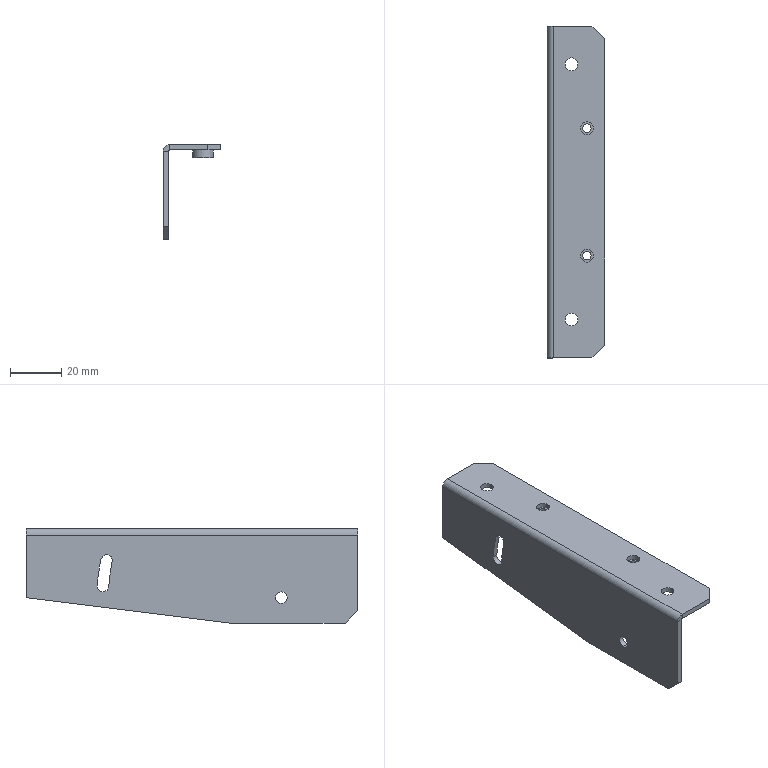Part | SolidWorks | features ICE 3, Chamfer 2, Cut 2, FlatPattern 1, HoleWzd 1, SMBaseFlange 1, SheetMetal 1 | 1 solid | 45 faces | box 22.5 x 130 x 37 mm | volume 13846 mm3 | cylinder 25 | plane 20 | commonest cylinder face diameters 5 x9 4.5 x5 3.3 x4 8 x4 1 x1 135.5 x1
STEP:
#1=CARTESIAN_POINT('',(15.15,40.,-3.));
#2=VERTEX_POINT('',#1);
#3=CARTESIAN_POINT('',(11.85,40.,-3.));
#4=VERTEX_POINT('',#3);
#5=CARTESIAN_POINT('',(13.5,40.,-3.));
#6=DIRECTION('',(0.,0.,-1.));
#7=DIRECTION('',(-1.,0.,0.));
#8=AXIS2_PLACEMENT_3D('',#5,#6,#7);
#9=CIRCLE('',#8,1.65);
#10=EDGE_CURVE('',#2,#4,#9,.T.);
#11=ORIENTED_EDGE('',*,*,#10,.T.);
#12=CARTESIAN_POINT('',(11.85,40.,0.));
#13=VERTEX_POINT('',#12);
#14=CARTESIAN_POINT('',(11.85,40.,0.));
#15=DIRECTION('',(0.,0.,1.));
#16=VECTOR('',#15,1000.);
#17=LINE('',#14,#16);
#18=EDGE_CURVE('',#4,#13,#17,.T.);
#19=ORIENTED_EDGE('',*,*,#18,.T.);
#20=CARTESIAN_POINT('',(15.15,40.,0.));
#21=VERTEX_POINT('',#20);
#22=CARTESIAN_POINT('',(13.5,40.,0.));
#23=DIRECTION('',(0.,0.,1.));
#24=DIRECTION('',(1.,0.,0.));
#25=AXIS2_PLACEMENT_3D('',#22,#23,#24);
#26=CIRCLE('',#25,1.65);
#27=EDGE_CURVE('',#13,#21,#26,.T.);
#28=ORIENTED_EDGE('',*,*,#27,.T.);
#29=CARTESIAN_POINT('',(15.15,40.,0.));
#30=DIRECTION('',(0.,0.,1.));
#31=VECTOR('',#30,1000.);
#32=LINE('',#29,#31);
#33=EDGE_CURVE('',#2,#21,#32,.T.);
#34=ORIENTED_EDGE('',*,*,#33,.F.);
#35=EDGE_LOOP('',(#11,#19,#28,#34));
#36=FACE_OUTER_BOUND('',#35,.T.);
#37=CARTESIAN_POINT('',(13.5,40.,0.));
#38=DIRECTION('',(0.,0.,1.));
#39=DIRECTION('',(1.,0.,0.));
#40=AXIS2_PLACEMENT_3D('',#37,#38,#39);
#41=CYLINDRICAL_SURFACE('',#40,1.65);
#42=ADVANCED_FACE('',(#36),#41,.F.);
#43=CARTESIAN_POINT('',(15.15,90.,-3.));
#44=VERTEX_POINT('',#43);
#45=CARTESIAN_POINT('',(11.85,90.,-3.));
#46=VERTEX_POINT('',#45);
#47=CARTESIAN_POINT('',(13.5,90.,-3.));
#48=DIRECTION('',(0.,0.,-1.));
#49=DIRECTION('',(-1.,0.,0.));
#50=AXIS2_PLACEMENT_3D('',#47,#48,#49);
#51=CIRCLE('',#50,1.65);
#52=EDGE_CURVE('',#44,#46,#51,.T.);
#53=ORIENTED_EDGE('',*,*,#52,.T.);
#54=CARTESIAN_POINT('',(11.85,90.,0.));
#55=VERTEX_POINT('',#54);
#56=CARTESIAN_POINT('',(11.85,90.,0.));
#57=DIRECTION('',(0.,0.,1.));
#58=VECTOR('',#57,1000.);
#59=LINE('',#56,#58);
#60=EDGE_CURVE('',#46,#55,#59,.T.);
#61=ORIENTED_EDGE('',*,*,#60,.T.);
#62=CARTESIAN_POINT('',(15.15,90.,0.));
#63=VERTEX_POINT('',#62);
#64=CARTESIAN_POINT('',(13.5,90.,0.));
#65=DIRECTION('',(0.,0.,1.));
#66=DIRECTION('',(1.,0.,0.));
#67=AXIS2_PLACEMENT_3D('',#64,#65,#66);
#68=CIRCLE('',#67,1.65);
#69=EDGE_CURVE('',#55,#63,#68,.T.);
#70=ORIENTED_EDGE('',*,*,#69,.T.);
#71=CARTESIAN_POINT('',(15.15,90.,0.));
#72=DIRECTION('',(0.,0.,1.));
#73=VECTOR('',#72,1000.);
#74=LINE('',#71,#73);
#75=EDGE_CURVE('',#44,#63,#74,.T.);
#76=ORIENTED_EDGE('',*,*,#75,.F.);
#77=EDGE_LOOP('',(#53,#61,#70,#76));
#78=FACE_OUTER_BOUND('',#77,.T.);
#79=CARTESIAN_POINT('',(13.5,90.,0.));
#80=DIRECTION('',(0.,0.,1.));
#81=DIRECTION('',(1.,0.,0.));
#82=AXIS2_PLACEMENT_3D('',#79,#80,#81);
#83=CYLINDRICAL_SURFACE('',#82,1.65);
#84=ADVANCED_FACE('',(#78),#83,.F.);
#85=CARTESIAN_POINT('',(9.5,90.,-3.));
#86=VERTEX_POINT('',#85);
#87=CARTESIAN_POINT('',(17.5,90.,-3.));
#88=VERTEX_POINT('',#87);
#89=CARTESIAN_POINT('',(13.5,90.,-3.));
#90=DIRECTION('',(0.,0.,-1.));
#91=DIRECTION('',(-1.,0.,0.));
#92=AXIS2_PLACEMENT_3D('',#89,#90,#91);
#93=CIRCLE('',#92,4.);
#94=EDGE_CURVE('',#86,#88,#93,.T.);
#95=ORIENTED_EDGE('',*,*,#94,.F.);
#96=CARTESIAN_POINT('',(9.5,90.,0.));
#97=VERTEX_POINT('',#96);
#98=CARTESIAN_POINT('',(9.5,90.,-3.));
#99=DIRECTION('',(0.,0.,1.));
#100=VECTOR('',#99,1000.);
#101=LINE('',#98,#100);
#102=EDGE_CURVE('',#86,#97,#101,.T.);
#103=ORIENTED_EDGE('',*,*,#102,.T.);
#104=CARTESIAN_POINT('',(17.5,90.,0.));
#105=VERTEX_POINT('',#104);
#106=CARTESIAN_POINT('',(13.5,90.,0.));
#107=DIRECTION('',(0.,0.,-1.));
#108=DIRECTION('',(-1.,0.,0.));
#109=AXIS2_PLACEMENT_3D('',#106,#107,#108);
#110=CIRCLE('',#109,4.);
#111=EDGE_CURVE('',#97,#105,#110,.T.);
#112=ORIENTED_EDGE('',*,*,#111,.T.);
#113=CARTESIAN_POINT('',(17.5,90.,-3.));
#114=DIRECTION('',(0.,0.,1.));
#115=VECTOR('',#114,1000.);
#116=LINE('',#113,#115);
#117=EDGE_CURVE('',#88,#105,#116,.T.);
#118=ORIENTED_EDGE('',*,*,#117,.F.);
#119=EDGE_LOOP('',(#95,#103,#112,#118));
#120=FACE_OUTER_BOUND('',#119,.T.);
#121=CARTESIAN_POINT('',(13.5,90.,-3.));
#122=DIRECTION('',(0.,0.,1.));
#123=DIRECTION('',(1.,0.,0.));
#124=AXIS2_PLACEMENT_3D('',#121,#122,#123);
#125=CYLINDRICAL_SURFACE('',#124,4.);
#126=ADVANCED_FACE('',(#120),#125,.T.);
#127=CARTESIAN_POINT('',(9.5,40.,-3.));
#128=VERTEX_POINT('',#127);
#129=CARTESIAN_POINT('',(17.5,40.,-3.));
#130=VERTEX_POINT('',#129);
#131=CARTESIAN_POINT('',(13.5,40.,-3.));
#132=DIRECTION('',(0.,0.,-1.));
#133=DIRECTION('',(-1.,0.,0.));
#134=AXIS2_PLACEMENT_3D('',#131,#132,#133);
#135=CIRCLE('',#134,4.);
#136=EDGE_CURVE('',#128,#130,#135,.T.);
#137=ORIENTED_EDGE('',*,*,#136,.F.);
#138=CARTESIAN_POINT('',(9.5,40.,0.));
#139=VERTEX_POINT('',#138);
#140=CARTESIAN_POINT('',(9.5,40.,-3.));
#141=DIRECTION('',(0.,0.,1.));
#142=VECTOR('',#141,1000.);
#143=LINE('',#140,#142);
#144=EDGE_CURVE('',#128,#139,#143,.T.);
#145=ORIENTED_EDGE('',*,*,#144,.T.);
#146=CARTESIAN_POINT('',(17.5,40.,0.));
#147=VERTEX_POINT('',#146);
#148=CARTESIAN_POINT('',(13.5,40.,0.));
#149=DIRECTION('',(0.,0.,-1.));
#150=DIRECTION('',(-1.,0.,0.));
#151=AXIS2_PLACEMENT_3D('',#148,#149,#150);
#152=CIRCLE('',#151,4.);
#153=EDGE_CURVE('',#139,#147,#152,.T.);
#154=ORIENTED_EDGE('',*,*,#153,.T.);
#155=CARTESIAN_POINT('',(17.5,40.,-3.));
#156=DIRECTION('',(0.,0.,1.));
#157=VECTOR('',#156,1000.);
#158=LINE('',#155,#157);
#159=EDGE_CURVE('',#130,#147,#158,.T.);
#160=ORIENTED_EDGE('',*,*,#159,.F.);
#161=EDGE_LOOP('',(#137,#145,#154,#160));
#162=FACE_OUTER_BOUND('',#161,.T.);
#163=CARTESIAN_POINT('',(13.5,40.,-3.));
#164=DIRECTION('',(0.,0.,1.));
#165=DIRECTION('',(1.,0.,0.));
#166=AXIS2_PLACEMENT_3D('',#163,#164,#165);
#167=CYLINDRICAL_SURFACE('',#166,4.);
#168=ADVANCED_FACE('',(#162),#167,.T.);
#169=CARTESIAN_POINT('',(16.,40.,2.));
#170=VERTEX_POINT('',#169);
#171=CARTESIAN_POINT('',(11.,40.,2.));
#172=VERTEX_POINT('',#171);
#173=CARTESIAN_POINT('',(13.5,40.,2.));
#174=DIRECTION('',(0.,0.,-1.));
#175=DIRECTION('',(-1.,0.,0.));
#176=AXIS2_PLACEMENT_3D('',#173,#174,#175);
#177=CIRCLE('',#176,2.5);
#178=EDGE_CURVE('',#170,#172,#177,.T.);
#179=ORIENTED_EDGE('',*,*,#178,.F.);
#180=CARTESIAN_POINT('',(16.,40.,0.));
#181=VERTEX_POINT('',#180);
#182=CARTESIAN_POINT('',(16.,40.,5.));
#183=DIRECTION('',(0.,0.,-1.));
#184=VECTOR('',#183,1000.);
#185=LINE('',#182,#184);
#186=EDGE_CURVE('',#170,#181,#185,.T.);
#187=ORIENTED_EDGE('',*,*,#186,.T.);
#188=CARTESIAN_POINT('',(11.,40.,0.));
#189=VERTEX_POINT('',#188);
#190=CARTESIAN_POINT('',(13.5,40.,0.));
#191=DIRECTION('',(0.,0.,1.));
#192=DIRECTION('',(-1.,0.,0.));
#193=AXIS2_PLACEMENT_3D('',#190,#191,#192);
#194=CIRCLE('',#193,2.5);
#195=EDGE_CURVE('',#189,#181,#194,.T.);
#196=ORIENTED_EDGE('',*,*,#195,.F.);
#197=CARTESIAN_POINT('',(11.,40.,5.));
#198=DIRECTION('',(0.,0.,-1.));
#199=VECTOR('',#198,1000.);
#200=LINE('',#197,#199);
#201=EDGE_CURVE('',#172,#189,#200,.T.);
#202=ORIENTED_EDGE('',*,*,#201,.F.);
#203=EDGE_LOOP('',(#179,#187,#196,#202));
#204=FACE_OUTER_BOUND('',#203,.T.);
#205=CARTESIAN_POINT('',(13.5,40.,5.));
#206=DIRECTION('',(0.,0.,-1.));
#207=DIRECTION('',(-1.,0.,0.));
#208=AXIS2_PLACEMENT_3D('',#205,#206,#207);
#209=CYLINDRICAL_SURFACE('',#208,2.5);
#210=ADVANCED_FACE('',(#204),#209,.F.);
#211=CARTESIAN_POINT('',(16.,90.,2.));
#212=VERTEX_POINT('',#211);
#213=CARTESIAN_POINT('',(11.,90.,2.));
#214=VERTEX_POINT('',#213);
#215=CARTESIAN_POINT('',(13.5,90.,2.));
#216=DIRECTION('',(0.,0.,-1.));
#217=DIRECTION('',(-1.,0.,0.));
#218=AXIS2_PLACEMENT_3D('',#215,#216,#217);
#219=CIRCLE('',#218,2.5);
#220=EDGE_CURVE('',#212,#214,#219,.T.);
#221=ORIENTED_EDGE('',*,*,#220,.F.);
#222=CARTESIAN_POINT('',(16.,90.,0.));
#223=VERTEX_POINT('',#222);
#224=CARTESIAN_POINT('',(16.,90.,5.));
#225=DIRECTION('',(0.,0.,-1.));
#226=VECTOR('',#225,1000.);
#227=LINE('',#224,#226);
#228=EDGE_CURVE('',#212,#223,#227,.T.);
#229=ORIENTED_EDGE('',*,*,#228,.T.);
#230=CARTESIAN_POINT('',(11.,90.,0.));
#231=VERTEX_POINT('',#230);
#232=CARTESIAN_POINT('',(13.5,90.,0.));
#233=DIRECTION('',(0.,0.,1.));
#234=DIRECTION('',(-1.,0.,0.));
#235=AXIS2_PLACEMENT_3D('',#232,#233,#234);
#236=CIRCLE('',#235,2.5);
#237=EDGE_CURVE('',#231,#223,#236,.T.);
#238=ORIENTED_EDGE('',*,*,#237,.F.);
#239=CARTESIAN_POINT('',(11.,90.,5.));
#240=DIRECTION('',(0.,0.,-1.));
#241=VECTOR('',#240,1000.);
#242=LINE('',#239,#241);
#243=EDGE_CURVE('',#214,#231,#242,.T.);
#244=ORIENTED_EDGE('',*,*,#243,.F.);
#245=EDGE_LOOP('',(#221,#229,#238,#244));
#246=FACE_OUTER_BOUND('',#245,.T.);
#247=CARTESIAN_POINT('',(13.5,90.,5.));
#248=DIRECTION('',(0.,0.,-1.));
#249=DIRECTION('',(-1.,0.,0.));
#250=AXIS2_PLACEMENT_3D('',#247,#248,#249);
#251=CYLINDRICAL_SURFACE('',#250,2.5);
#252=ADVANCED_FACE('',(#246),#251,.F.);
#253=CARTESIAN_POINT('',(0.,100.671,-9.978));
#254=VERTEX_POINT('',#253);
#255=CARTESIAN_POINT('',(0.,98.47,-8.196));
#256=VERTEX_POINT('',#255);
#257=CARTESIAN_POINT('',(0.,98.47,-10.446));
#258=DIRECTION('',(1.,0.,0.));
#259=DIRECTION('',(0.,0.,-1.));
#260=AXIS2_PLACEMENT_3D('',#257,#258,#259);
#261=CIRCLE('',#260,2.25);
#262=EDGE_CURVE('',#254,#256,#261,.T.);
#263=ORIENTED_EDGE('',*,*,#262,.T.);
#264=CARTESIAN_POINT('',(-2.,98.47,-8.196));
#265=VERTEX_POINT('',#264);
#266=CARTESIAN_POINT('',(8.,98.47,-8.196));
#267=DIRECTION('',(-1.,0.,0.));
#268=VECTOR('',#267,1000.);
#269=LINE('',#266,#268);
#270=EDGE_CURVE('',#256,#265,#269,.T.);
#271=ORIENTED_EDGE('',*,*,#270,.T.);
#272=CARTESIAN_POINT('',(-2.,100.671,-9.978));
#273=VERTEX_POINT('',#272);
#274=CARTESIAN_POINT('',(-2.,98.47,-10.446));
#275=DIRECTION('',(-1.,0.,0.));
#276=DIRECTION('',(0.,0.,1.));
#277=AXIS2_PLACEMENT_3D('',#274,#275,#276);
#278=CIRCLE('',#277,2.25);
#279=EDGE_CURVE('',#265,#273,#278,.T.);
#280=ORIENTED_EDGE('',*,*,#279,.T.);
#281=CARTESIAN_POINT('',(8.,100.671,-9.978));
#282=DIRECTION('',(-1.,0.,0.));
#283=VECTOR('',#282,1000.);
#284=LINE('',#281,#283);
#285=EDGE_CURVE('',#254,#273,#284,.T.);
#286=ORIENTED_EDGE('',*,*,#285,.F.);
#287=EDGE_LOOP('',(#263,#271,#280,#286));
#288=FACE_OUTER_BOUND('',#287,.T.);
#289=CARTESIAN_POINT('',(8.,98.47,-10.446));
#290=DIRECTION('',(-1.,0.,0.));
#291=DIRECTION('',(0.,0.,1.));
#292=AXIS2_PLACEMENT_3D('',#289,#290,#291);
#293=CYLINDRICAL_SURFACE('',#292,2.25);
#294=ADVANCED_FACE('',(#288),#293,.F.);
#295=CARTESIAN_POINT('',(-2.,30.,-22.75));
#296=VERTEX_POINT('',#295);
#297=CARTESIAN_POINT('',(-2.,30.,-27.25));
#298=VERTEX_POINT('',#297);
#299=CARTESIAN_POINT('',(-2.,30.,-25.));
#300=DIRECTION('',(1.,0.,0.));
#301=DIRECTION('',(0.,0.,-1.));
#302=AXIS2_PLACEMENT_3D('',#299,#300,#301);
#303=CIRCLE('',#302,2.25);
#304=EDGE_CURVE('',#296,#298,#303,.T.);
#305=ORIENTED_EDGE('',*,*,#304,.F.);
#306=CARTESIAN_POINT('',(0.,30.,-22.75));
#307=VERTEX_POINT('',#306);
#308=CARTESIAN_POINT('',(-10.,30.,-22.75));
#309=DIRECTION('',(1.,0.,0.));
#310=VECTOR('',#309,1000.);
#311=LINE('',#308,#310);
#312=EDGE_CURVE('',#296,#307,#311,.T.);
#313=ORIENTED_EDGE('',*,*,#312,.T.);
#314=CARTESIAN_POINT('',(0.,30.,-27.25));
#315=VERTEX_POINT('',#314);
#316=CARTESIAN_POINT('',(0.,30.,-25.));
#317=DIRECTION('',(1.,0.,0.));
#318=DIRECTION('',(0.,0.,-1.));
#319=AXIS2_PLACEMENT_3D('',#316,#317,#318);
#320=CIRCLE('',#319,2.25);
#321=EDGE_CURVE('',#307,#315,#320,.T.);
#322=ORIENTED_EDGE('',*,*,#321,.T.);
#323=CARTESIAN_POINT('',(-10.,30.,-27.25));
#324=DIRECTION('',(1.,0.,0.));
#325=VECTOR('',#324,1000.);
#326=LINE('',#323,#325);
#327=EDGE_CURVE('',#298,#315,#326,.T.);
#328=ORIENTED_EDGE('',*,*,#327,.F.);
#329=EDGE_LOOP('',(#305,#313,#322,#328));
#330=FACE_OUTER_BOUND('',#329,.T.);
#331=CARTESIAN_POINT('',(-10.,30.,-25.));
#332=DIRECTION('',(1.,0.,0.));
#333=DIRECTION('',(0.,0.,-1.));
#334=AXIS2_PLACEMENT_3D('',#331,#332,#333);
#335=CYLINDRICAL_SURFACE('',#334,2.25);
#336=ADVANCED_FACE('',(#330),#335,.F.);
#337=CARTESIAN_POINT('',(10.,15.,0.));
#338=VERTEX_POINT('',#337);
#339=CARTESIAN_POINT('',(5.,15.,0.));
#340=VERTEX_POINT('',#339);
#341=CARTESIAN_POINT('',(7.5,15.,0.));
#342=DIRECTION('',(0.,0.,-1.));
#343=DIRECTION('',(-1.,0.,0.));
#344=AXIS2_PLACEMENT_3D('',#341,#342,#343);
#345=CIRCLE('',#344,2.5);
#346=EDGE_CURVE('',#338,#340,#345,.T.);
#347=ORIENTED_EDGE('',*,*,#346,.T.);
#348=CARTESIAN_POINT('',(5.,15.,2.));
#349=VERTEX_POINT('',#348);
#350=CARTESIAN_POINT('',(5.,15.,-8.));
#351=DIRECTION('',(0.,0.,1.));
#352=VECTOR('',#351,1000.);
#353=LINE('',#350,#352);
#354=EDGE_CURVE('',#340,#349,#353,.T.);
#355=ORIENTED_EDGE('',*,*,#354,.T.);
#356=CARTESIAN_POINT('',(10.,15.,2.));
#357=VERTEX_POINT('',#356);
#358=CARTESIAN_POINT('',(7.5,15.,2.));
#359=DIRECTION('',(0.,0.,1.));
#360=DIRECTION('',(1.,0.,0.));
#361=AXIS2_PLACEMENT_3D('',#358,#359,#360);
#362=CIRCLE('',#361,2.5);
#363=EDGE_CURVE('',#349,#357,#362,.T.);
#364=ORIENTED_EDGE('',*,*,#363,.T.);
#365=CARTESIAN_POINT('',(10.,15.,-8.));
#366=DIRECTION('',(0.,0.,1.));
#367=VECTOR('',#366,1000.);
#368=LINE('',#365,#367);
#369=EDGE_CURVE('',#338,#357,#368,.T.);
#370=ORIENTED_EDGE('',*,*,#369,.F.);
#371=EDGE_LOOP('',(#347,#355,#364,#370));
#372=FACE_OUTER_BOUND('',#371,.T.);
#373=CARTESIAN_POINT('',(7.5,15.,-8.));
#374=DIRECTION('',(0.,0.,1.));
#375=DIRECTION('',(1.,0.,0.));
#376=AXIS2_PLACEMENT_3D('',#373,#374,#375);
#377=CYLINDRICAL_SURFACE('',#376,2.5);
#378=ADVANCED_FACE('',(#372),#377,.F.);
#379=CARTESIAN_POINT('',(10.,115.,0.));
#380=VERTEX_POINT('',#379);
#381=CARTESIAN_POINT('',(5.,115.,0.));
#382=VERTEX_POINT('',#381);
#383=CARTESIAN_POINT('',(7.5,115.,0.));
#384=DIRECTION('',(0.,0.,-1.));
#385=DIRECTION('',(-1.,0.,0.));
#386=AXIS2_PLACEMENT_3D('',#383,#384,#385);
#387=CIRCLE('',#386,2.5);
#388=EDGE_CURVE('',#380,#382,#387,.T.);
#389=ORIENTED_EDGE('',*,*,#388,.T.);
#390=CARTESIAN_POINT('',(5.,115.,2.));
#391=VERTEX_POINT('',#390);
#392=CARTESIAN_POINT('',(5.,115.,-8.));
#393=DIRECTION('',(0.,0.,1.));
#394=VECTOR('',#393,1000.);
#395=LINE('',#392,#394);
#396=EDGE_CURVE('',#382,#391,#395,.T.);
#397=ORIENTED_EDGE('',*,*,#396,.T.);
#398=CARTESIAN_POINT('',(10.,115.,2.));
#399=VERTEX_POINT('',#398);
#400=CARTESIAN_POINT('',(7.5,115.,2.));
#401=DIRECTION('',(0.,0.,1.));
#402=DIRECTION('',(1.,0.,0.));
#403=AXIS2_PLACEMENT_3D('',#400,#401,#402);
#404=CIRCLE('',#403,2.5);
#405=EDGE_CURVE('',#391,#399,#404,.T.);
#406=ORIENTED_EDGE('',*,*,#405,.T.);
#407=CARTESIAN_POINT('',(10.,115.,-8.));
#408=DIRECTION('',(0.,0.,1.));
#409=VECTOR('',#408,1000.);
#410=LINE('',#407,#409);
#411=EDGE_CURVE('',#380,#399,#410,.T.);
#412=ORIENTED_EDGE('',*,*,#411,.F.);
#413=EDGE_LOOP('',(#389,#397,#406,#412));
#414=FACE_OUTER_BOUND('',#413,.T.);
#415=CARTESIAN_POINT('',(7.5,115.,-8.));
#416=DIRECTION('',(0.,0.,1.));
#417=DIRECTION('',(1.,0.,0.));
#418=AXIS2_PLACEMENT_3D('',#415,#416,#417);
#419=CYLINDRICAL_SURFACE('',#418,2.5);
#420=ADVANCED_FACE('',(#414),#419,.F.);
#421=CARTESIAN_POINT('',(13.5,40.,0.));
#422=DIRECTION('',(0.,0.,-1.));
#423=DIRECTION('',(-1.,0.,0.));
#424=AXIS2_PLACEMENT_3D('',#421,#422,#423);
#425=CIRCLE('',#424,4.);
#426=EDGE_CURVE('',#147,#139,#425,.T.);
#427=ORIENTED_EDGE('',*,*,#426,.F.);
#428=ORIENTED_EDGE('',*,*,#153,.F.);
#429=EDGE_LOOP('',(#427,#428));
#430=FACE_BOUND('',#429,.T.);
#431=ORIENTED_EDGE('',*,*,#346,.F.);
#432=CARTESIAN_POINT('',(7.5,15.,0.));
#433=DIRECTION('',(0.,0.,-1.));
#434=DIRECTION('',(-1.,0.,0.));
#435=AXIS2_PLACEMENT_3D('',#432,#433,#434);
#436=CIRCLE('',#435,2.5);
#437=EDGE_CURVE('',#340,#338,#436,.T.);
#438=ORIENTED_EDGE('',*,*,#437,.F.);
#439=EDGE_LOOP('',(#431,#438));
#440=FACE_BOUND('',#439,.T.);
#441=ORIENTED_EDGE('',*,*,#388,.F.);
#442=CARTESIAN_POINT('',(7.5,115.,0.));
#443=DIRECTION('',(0.,0.,-1.));
#444=DIRECTION('',(-1.,0.,0.));
#445=AXIS2_PLACEMENT_3D('',#442,#443,#444);
#446=CIRCLE('',#445,2.5);
#447=EDGE_CURVE('',#382,#380,#446,.T.);
#448=ORIENTED_EDGE('',*,*,#447,.F.);
#449=EDGE_LOOP('',(#441,#448));
#450=FACE_BOUND('',#449,.T.);
#451=CARTESIAN_POINT('',(20.5,125.,0.));
#452=VERTEX_POINT('',#451);
#453=CARTESIAN_POINT('',(20.5,5.,0.));
#454=VERTEX_POINT('',#453);
#455=CARTESIAN_POINT('',(20.5,130.,0.));
#456=DIRECTION('',(0.,-1.,0.));
#457=VECTOR('',#456,1000.);
#458=LINE('',#455,#457);
#459=EDGE_CURVE('',#452,#454,#458,.T.);
#460=ORIENTED_EDGE('',*,*,#459,.T.);
#461=CARTESIAN_POINT('',(15.5,0.,0.));
#462=VERTEX_POINT('',#461);
#463=CARTESIAN_POINT('',(72.75,57.25,0.));
#464=DIRECTION('',(-0.7071,-0.7071,0.));
#465=VECTOR('',#464,1000.);
#466=LINE('',#463,#465);
#467=EDGE_CURVE('',#454,#462,#466,.T.);
#468=ORIENTED_EDGE('',*,*,#467,.T.);
#469=CARTESIAN_POINT('',(0.5,0.,0.));
#470=VERTEX_POINT('',#469);
#471=CARTESIAN_POINT('',(0.,0.,0.));
#472=DIRECTION('',(1.,0.,0.));
#473=VECTOR('',#472,1000.);
#474=LINE('',#471,#473);
#475=EDGE_CURVE('',#470,#462,#474,.T.);
#476=ORIENTED_EDGE('',*,*,#475,.F.);
#477=CARTESIAN_POINT('',(0.5,130.,0.));
#478=VERTEX_POINT('',#477);
#479=CARTESIAN_POINT('',(0.5,130.,0.));
#480=DIRECTION('',(0.,-1.,0.));
#481=VECTOR('',#480,1000.);
#482=LINE('',#479,#481);
#483=EDGE_CURVE('',#478,#470,#482,.T.);
#484=ORIENTED_EDGE('',*,*,#483,.F.);
#485=CARTESIAN_POINT('',(15.5,130.,0.));
#486=VERTEX_POINT('',#485);
#487=CARTESIAN_POINT('',(0.,130.,0.));
#488=DIRECTION('',(1.,0.,0.));
#489=VECTOR('',#488,1000.);
#490=LINE('',#487,#489);
#491=EDGE_CURVE('',#478,#486,#490,.T.);
#492=ORIENTED_EDGE('',*,*,#491,.T.);
#493=CARTESIAN_POINT('',(7.75,137.75,0.));
#494=DIRECTION('',(0.7071,-0.7071,0.));
#495=VECTOR('',#494,1000.);
#496=LINE('',#493,#495);
#497=EDGE_CURVE('',#486,#452,#496,.T.);
#498=ORIENTED_EDGE('',*,*,#497,.T.);
#499=EDGE_LOOP('',(#460,#468,#476,#484,#492,#498));
#500=FACE_OUTER_BOUND('',#499,.T.);
#501=CARTESIAN_POINT('',(13.5,90.,0.));
#502=DIRECTION('',(0.,0.,-1.));
#503=DIRECTION('',(-1.,0.,0.));
#504=AXIS2_PLACEMENT_3D('',#501,#502,#503);
#505=CIRCLE('',#504,4.);
#506=EDGE_CURVE('',#105,#97,#505,.T.);
#507=ORIENTED_EDGE('',*,*,#506,.F.);
#508=ORIENTED_EDGE('',*,*,#111,.F.);
#509=EDGE_LOOP('',(#507,#508));
#510=FACE_BOUND('',#509,.T.);
#511=CARTESIAN_POINT('',(0.,130.,0.));
#512=DIRECTION('',(0.,0.,-1.));
#513=DIRECTION('',(-1.,0.,0.));
#514=AXIS2_PLACEMENT_3D('',#511,#512,#513);
#515=PLANE('',#514);
#516=ADVANCED_FACE('',(#430,#440,#450,#500,#510),#515,.T.);
#517=CARTESIAN_POINT('',(0.5,130.,2.));
#518=VERTEX_POINT('',#517);
#519=CARTESIAN_POINT('',(0.5,130.,0.));
#520=DIRECTION('',(0.,0.,1.));
#521=VECTOR('',#520,1000.);
#522=LINE('',#519,#521);
#523=EDGE_CURVE('',#478,#518,#522,.T.);
#524=ORIENTED_EDGE('',*,*,#523,.F.);
#525=CARTESIAN_POINT('',(0.,130.,-0.5));
#526=VERTEX_POINT('',#525);
#527=CARTESIAN_POINT('',(0.5,130.,-0.5));
#528=DIRECTION('',(0.,1.,0.));
#529=DIRECTION('',(0.,0.,-1.));
#530=AXIS2_PLACEMENT_3D('',#527,#528,#529);
#531=CIRCLE('',#530,0.5);
#532=EDGE_CURVE('',#526,#478,#531,.T.);
#533=ORIENTED_EDGE('',*,*,#532,.F.);
#534=CARTESIAN_POINT('',(-2.,130.,-0.5));
#535=VERTEX_POINT('',#534);
#536=CARTESIAN_POINT('',(-2.,130.,-0.5));
#537=DIRECTION('',(1.,0.,0.));
#538=VECTOR('',#537,1000.);
#539=LINE('',#536,#538);
#540=EDGE_CURVE('',#535,#526,#539,.T.);
#541=ORIENTED_EDGE('',*,*,#540,.F.);
#542=CARTESIAN_POINT('',(0.5,130.,-0.5));
#543=DIRECTION('',(0.,1.,0.));
#544=DIRECTION('',(1.,0.,0.));
#545=AXIS2_PLACEMENT_3D('',#542,#543,#544);
#546=CIRCLE('',#545,2.5);
#547=EDGE_CURVE('',#535,#518,#546,.T.);
#548=ORIENTED_EDGE('',*,*,#547,.T.);
#549=EDGE_LOOP('',(#524,#533,#541,#548));
#550=FACE_OUTER_BOUND('',#549,.T.);
#551=CARTESIAN_POINT('',(0.5,130.,0.));
#552=DIRECTION('',(0.,1.,0.));
#553=DIRECTION('',(0.,0.,1.));
#554=AXIS2_PLACEMENT_3D('',#551,#552,#553);
#555=PLANE('',#554);
#556=ADVANCED_FACE('',(#550),#555,.T.);
#557=CARTESIAN_POINT('',(15.5,130.,2.));
#558=VERTEX_POINT('',#557);
#559=CARTESIAN_POINT('',(0.,130.,2.));
#560=DIRECTION('',(1.,0.,0.));
#561=VECTOR('',#560,1000.);
#562=LINE('',#559,#561);
#563=EDGE_CURVE('',#518,#558,#562,.T.);
#564=ORIENTED_EDGE('',*,*,#563,.T.);
#565=CARTESIAN_POINT('',(15.5,130.,-0.5));
#566=DIRECTION('',(0.,0.,-1.));
#567=VECTOR('',#566,1000.);
#568=LINE('',#565,#567);
#569=EDGE_CURVE('',#558,#486,#568,.T.);
#570=ORIENTED_EDGE('',*,*,#569,.T.);
#571=ORIENTED_EDGE('',*,*,#491,.F.);
#572=ORIENTED_EDGE('',*,*,#523,.T.);
#573=EDGE_LOOP('',(#564,#570,#571,#572));
#574=FACE_OUTER_BOUND('',#573,.T.);
#575=CARTESIAN_POINT('',(-2.,130.,-0.5));
#576=DIRECTION('',(0.,1.,0.));
#577=DIRECTION('',(0.,0.,1.));
#578=AXIS2_PLACEMENT_3D('',#575,#576,#577);
#579=PLANE('',#578);
#580=ADVANCED_FACE('',(#574),#579,.T.);
#581=CARTESIAN_POINT('',(0.,0.,-0.5));
#582=VERTEX_POINT('',#581);
#583=CARTESIAN_POINT('',(-2.,0.,-0.5));
#584=VERTEX_POINT('',#583);
#585=CARTESIAN_POINT('',(0.,0.,-0.5));
#586=DIRECTION('',(-1.,0.,0.));
#587=VECTOR('',#586,1000.);
#588=LINE('',#585,#587);
#589=EDGE_CURVE('',#582,#584,#588,.T.);
#590=ORIENTED_EDGE('',*,*,#589,.F.);
#591=CARTESIAN_POINT('',(0.5,0.,-0.5));
#592=DIRECTION('',(0.,1.,0.));
#593=DIRECTION('',(0.,0.,-1.));
#594=AXIS2_PLACEMENT_3D('',#591,#592,#593);
#595=CIRCLE('',#594,0.5);
#596=EDGE_CURVE('',#582,#470,#595,.T.);
#597=ORIENTED_EDGE('',*,*,#596,.T.);
#598=CARTESIAN_POINT('',(0.5,0.,2.));
#599=VERTEX_POINT('',#598);
#600=CARTESIAN_POINT('',(0.5,0.,2.));
#601=DIRECTION('',(0.,0.,-1.));
#602=VECTOR('',#601,1000.);
#603=LINE('',#600,#602);
#604=EDGE_CURVE('',#599,#470,#603,.T.);
#605=ORIENTED_EDGE('',*,*,#604,.F.);
#606=CARTESIAN_POINT('',(0.5,0.,-0.5));
#607=DIRECTION('',(0.,1.,0.));
#608=DIRECTION('',(1.,0.,0.));
#609=AXIS2_PLACEMENT_3D('',#606,#607,#608);
#610=CIRCLE('',#609,2.5);
#611=EDGE_CURVE('',#584,#599,#610,.T.);
#612=ORIENTED_EDGE('',*,*,#611,.F.);
#613=EDGE_LOOP('',(#590,#597,#605,#612));
#614=FACE_OUTER_BOUND('',#613,.T.);
#615=CARTESIAN_POINT('',(0.,0.,-0.5));
#616=DIRECTION('',(0.,-1.,0.));
#617=DIRECTION('',(0.,0.,-1.));
#618=AXIS2_PLACEMENT_3D('',#615,#616,#617);
#619=PLANE('',#618);
#620=ADVANCED_FACE('',(#614),#619,.T.);
#621=CARTESIAN_POINT('',(-2.,0.,-30.));
#622=VERTEX_POINT('',#621);
#623=CARTESIAN_POINT('',(-2.,0.,0.));
#624=DIRECTION('',(0.,0.,1.));
#625=VECTOR('',#624,1000.);
#626=LINE('',#623,#625);
#627=EDGE_CURVE('',#622,#584,#626,.T.);
#628=ORIENTED_EDGE('',*,*,#627,.F.);
#629=CARTESIAN_POINT('',(0.,0.,-30.));
#630=VERTEX_POINT('',#629);
#631=CARTESIAN_POINT('',(0.5,0.,-30.));
#632=DIRECTION('',(1.,0.,0.));
#633=VECTOR('',#632,1000.);
#634=LINE('',#631,#633);
#635=EDGE_CURVE('',#622,#630,#634,.T.);
#636=ORIENTED_EDGE('',*,*,#635,.T.);
#637=CARTESIAN_POINT('',(0.,0.,0.));
#638=DIRECTION('',(0.,0.,1.));
#639=VECTOR('',#638,1000.);
#640=LINE('',#637,#639);
#641=EDGE_CURVE('',#630,#582,#640,.T.);
#642=ORIENTED_EDGE('',*,*,#641,.T.);
#643=ORIENTED_EDGE('',*,*,#589,.T.);
#644=EDGE_LOOP('',(#628,#636,#642,#643));
#645=FACE_OUTER_BOUND('',#644,.T.);
#646=CARTESIAN_POINT('',(0.5,0.,2.));
#647=DIRECTION('',(0.,-1.,0.));
#648=DIRECTION('',(0.,0.,-1.));
#649=AXIS2_PLACEMENT_3D('',#646,#647,#648);
#650=PLANE('',#649);
#651=ADVANCED_FACE('',(#645),#650,.T.);
#652=CARTESIAN_POINT('',(13.5,40.,2.));
#653=DIRECTION('',(0.,0.,-1.));
#654=DIRECTION('',(-1.,0.,0.));
#655=AXIS2_PLACEMENT_3D('',#652,#653,#654);
#656=CIRCLE('',#655,2.5);
#657=EDGE_CURVE('',#172,#170,#656,.T.);
#658=ORIENTED_EDGE('',*,*,#657,.T.);
#659=ORIENTED_EDGE('',*,*,#178,.T.);
#660=EDGE_LOOP('',(#658,#659));
#661=FACE_BOUND('',#660,.T.);
#662=CARTESIAN_POINT('',(13.5,90.,2.));
#663=DIRECTION('',(0.,0.,-1.));
#664=DIRECTION('',(-1.,0.,0.));
#665=AXIS2_PLACEMENT_3D('',#662,#663,#664);
#666=CIRCLE('',#665,2.5);
#667=EDGE_CURVE('',#214,#212,#666,.T.);
#668=ORIENTED_EDGE('',*,*,#667,.T.);
#669=ORIENTED_EDGE('',*,*,#220,.T.);
#670=EDGE_LOOP('',(#668,#669));
#671=FACE_BOUND('',#670,.T.);
#672=CARTESIAN_POINT('',(7.5,15.,2.));
#673=DIRECTION('',(0.,0.,1.));
#674=DIRECTION('',(1.,0.,0.));
#675=AXIS2_PLACEMENT_3D('',#672,#673,#674);
#676=CIRCLE('',#675,2.5);
#677=EDGE_CURVE('',#357,#349,#676,.T.);
#678=ORIENTED_EDGE('',*,*,#677,.F.);
#679=ORIENTED_EDGE('',*,*,#363,.F.);
#680=EDGE_LOOP('',(#678,#679));
#681=FACE_BOUND('',#680,.T.);
#682=CARTESIAN_POINT('',(7.5,115.,2.));
#683=DIRECTION('',(0.,0.,1.));
#684=DIRECTION('',(1.,0.,0.));
#685=AXIS2_PLACEMENT_3D('',#682,#683,#684);
#686=CIRCLE('',#685,2.5);
#687=EDGE_CURVE('',#399,#391,#686,.T.);
#688=ORIENTED_EDGE('',*,*,#687,.F.);
#689=ORIENTED_EDGE('',*,*,#405,.F.);
#690=EDGE_LOOP('',(#688,#689));
#691=FACE_BOUND('',#690,.T.);
#692=CARTESIAN_POINT('',(15.5,0.,2.));
#693=VERTEX_POINT('',#692);
#694=CARTESIAN_POINT('',(0.,0.,2.));
#695=DIRECTION('',(1.,0.,0.));
#696=VECTOR('',#695,1000.);
#697=LINE('',#694,#696);
#698=EDGE_CURVE('',#599,#693,#697,.T.);
#699=ORIENTED_EDGE('',*,*,#698,.T.);
#700=CARTESIAN_POINT('',(20.5,5.,2.));
#701=VERTEX_POINT('',#700);
#702=CARTESIAN_POINT('',(15.5,0.,2.));
#703=DIRECTION('',(0.7071,0.7071,0.));
#704=VECTOR('',#703,1000.);
#705=LINE('',#702,#704);
#706=EDGE_CURVE('',#693,#701,#705,.T.);
#707=ORIENTED_EDGE('',*,*,#706,.T.);
#708=CARTESIAN_POINT('',(20.5,125.,2.));
#709=VERTEX_POINT('',#708);
#710=CARTESIAN_POINT('',(20.5,130.,2.));
#711=DIRECTION('',(0.,-1.,0.));
#712=VECTOR('',#711,1000.);
#713=LINE('',#710,#712);
#714=EDGE_CURVE('',#709,#701,#713,.T.);
#715=ORIENTED_EDGE('',*,*,#714,.F.);
#716=CARTESIAN_POINT('',(20.5,125.,2.));
#717=DIRECTION('',(-0.7071,0.7071,0.));
#718=VECTOR('',#717,1000.);
#719=LINE('',#716,#718);
#720=EDGE_CURVE('',#709,#558,#719,.T.);
#721=ORIENTED_EDGE('',*,*,#720,.T.);
#722=ORIENTED_EDGE('',*,*,#563,.F.);
#723=CARTESIAN_POINT('',(0.5,130.,2.));
#724=DIRECTION('',(0.,-1.,0.));
#725=VECTOR('',#724,1000.);
#726=LINE('',#723,#725);
#727=EDGE_CURVE('',#518,#599,#726,.T.);
#728=ORIENTED_EDGE('',*,*,#727,.T.);
#729=EDGE_LOOP('',(#699,#707,#715,#721,#722,#728));
#730=FACE_OUTER_BOUND('',#729,.T.);
#731=CARTESIAN_POINT('',(0.,130.,2.));
#732=DIRECTION('',(0.,0.,-1.));
#733=DIRECTION('',(-1.,0.,0.));
#734=AXIS2_PLACEMENT_3D('',#731,#732,#733);
#735=PLANE('',#734);
#736=ADVANCED_FACE('',(#661,#671,#681,#691,#730),#735,.F.);
#737=ORIENTED_EDGE('',*,*,#714,.T.);
#738=CARTESIAN_POINT('',(20.5,5.,0.));
#739=DIRECTION('',(0.,0.,-1.));
#740=VECTOR('',#739,1000.);
#741=LINE('',#738,#740);
#742=EDGE_CURVE('',#701,#454,#741,.T.);
#743=ORIENTED_EDGE('',*,*,#742,.T.);
#744=ORIENTED_EDGE('',*,*,#459,.F.);
#745=CARTESIAN_POINT('',(20.5,125.,0.));
#746=DIRECTION('',(0.,0.,1.));
#747=VECTOR('',#746,1000.);
#748=LINE('',#745,#747);
#749=EDGE_CURVE('',#452,#709,#748,.T.);
#750=ORIENTED_EDGE('',*,*,#749,.T.);
#751=EDGE_LOOP('',(#737,#743,#744,#750));
#752=FACE_OUTER_BOUND('',#751,.T.);
#753=CARTESIAN_POINT('',(20.5,130.,0.));
#754=DIRECTION('',(1.,0.,0.));
#755=DIRECTION('',(0.,0.,-1.));
#756=AXIS2_PLACEMENT_3D('',#753,#754,#755);
#757=PLANE('',#756);
#758=ADVANCED_FACE('',(#752),#757,.T.);
#759=ORIENTED_EDGE('',*,*,#596,.F.);
#760=CARTESIAN_POINT('',(0.,130.,-0.5));
#761=DIRECTION('',(0.,-1.,0.));
#762=VECTOR('',#761,1000.);
#763=LINE('',#760,#762);
#764=EDGE_CURVE('',#526,#582,#763,.T.);
#765=ORIENTED_EDGE('',*,*,#764,.F.);
#766=ORIENTED_EDGE('',*,*,#532,.T.);
#767=ORIENTED_EDGE('',*,*,#483,.T.);
#768=EDGE_LOOP('',(#759,#765,#766,#767));
#769=FACE_OUTER_BOUND('',#768,.T.);
#770=CARTESIAN_POINT('',(0.5,130.,-0.5));
#771=DIRECTION('',(0.,-1.,0.));
#772=DIRECTION('',(0.,0.,-1.));
#773=AXIS2_PLACEMENT_3D('',#770,#771,#772);
#774=CYLINDRICAL_SURFACE('',#773,0.5);
#775=ADVANCED_FACE('',(#769),#774,.F.);
#776=CARTESIAN_POINT('',(0.,96.269,-10.914));
#777=VERTEX_POINT('',#776);
#778=CARTESIAN_POINT('',(0.,97.605,-20.569));
#779=VERTEX_POINT('',#778);
#780=CARTESIAN_POINT('',(0.,30.,-25.));
#781=DIRECTION('',(-1.,0.,0.));
#782=DIRECTION('',(0.,0.,-1.));
#783=AXIS2_PLACEMENT_3D('',#780,#781,#782);
#784=CIRCLE('',#783,67.75);
#785=EDGE_CURVE('',#777,#779,#784,.T.);
#786=ORIENTED_EDGE('',*,*,#785,.F.);
#787=CARTESIAN_POINT('',(0.,98.47,-10.446));
#788=DIRECTION('',(1.,0.,0.));
#789=DIRECTION('',(0.,0.,-1.));
#790=AXIS2_PLACEMENT_3D('',#787,#788,#789);
#791=CIRCLE('',#790,2.25);
#792=EDGE_CURVE('',#256,#777,#791,.T.);
#793=ORIENTED_EDGE('',*,*,#792,.F.);
#794=ORIENTED_EDGE('',*,*,#262,.F.);
#795=CARTESIAN_POINT('',(0.,102.095,-20.275));
#796=VERTEX_POINT('',#795);
#797=CARTESIAN_POINT('',(0.,30.,-25.));
#798=DIRECTION('',(1.,0.,0.));
#799=DIRECTION('',(0.,0.,-1.));
#800=AXIS2_PLACEMENT_3D('',#797,#798,#799);
#801=CIRCLE('',#800,72.25);
#802=EDGE_CURVE('',#796,#254,#801,.T.);
#803=ORIENTED_EDGE('',*,*,#802,.F.);
#804=CARTESIAN_POINT('',(0.,99.85,-20.422));
#805=DIRECTION('',(1.,0.,0.));
#806=DIRECTION('',(0.,0.,-1.));
#807=AXIS2_PLACEMENT_3D('',#804,#805,#806);
#808=CIRCLE('',#807,2.25);
#809=EDGE_CURVE('',#779,#796,#808,.T.);
#810=ORIENTED_EDGE('',*,*,#809,.F.);
#811=EDGE_LOOP('',(#786,#793,#794,#803,#810));
#812=FACE_BOUND('',#811,.T.);
#813=CARTESIAN_POINT('',(0.,30.,-25.));
#814=DIRECTION('',(1.,0.,0.));
#815=DIRECTION('',(0.,0.,-1.));
#816=AXIS2_PLACEMENT_3D('',#813,#814,#815);
#817=CIRCLE('',#816,2.25);
#818=EDGE_CURVE('',#315,#307,#817,.T.);
#819=ORIENTED_EDGE('',*,*,#818,.F.);
#820=ORIENTED_EDGE('',*,*,#321,.F.);
#821=EDGE_LOOP('',(#819,#820));
#822=FACE_BOUND('',#821,.T.);
#823=CARTESIAN_POINT('',(0.,50.,-35.));
#824=VERTEX_POINT('',#823);
#825=CARTESIAN_POINT('',(0.,5.,-35.));
#826=VERTEX_POINT('',#825);
#827=CARTESIAN_POINT('',(0.,130.,-35.));
#828=DIRECTION('',(0.,-1.,0.));
#829=VECTOR('',#828,1000.);
#830=LINE('',#827,#829);
#831=EDGE_CURVE('',#824,#826,#830,.T.);
#832=ORIENTED_EDGE('',*,*,#831,.F.);
#833=CARTESIAN_POINT('',(0.,130.,-25.));
#834=VERTEX_POINT('',#833);
#835=CARTESIAN_POINT('',(0.,133.077,-24.615));
#836=DIRECTION('',(0.,0.9923,0.124));
#837=VECTOR('',#836,1000.);
#838=LINE('',#835,#837);
#839=EDGE_CURVE('',#824,#834,#838,.T.);
#840=ORIENTED_EDGE('',*,*,#839,.T.);
#841=CARTESIAN_POINT('',(0.,130.,0.));
#842=DIRECTION('',(0.,0.,1.));
#843=VECTOR('',#842,1000.);
#844=LINE('',#841,#843);
#845=EDGE_CURVE('',#834,#526,#844,.T.);
#846=ORIENTED_EDGE('',*,*,#845,.T.);
#847=ORIENTED_EDGE('',*,*,#764,.T.);
#848=ORIENTED_EDGE('',*,*,#641,.F.);
#849=CARTESIAN_POINT('',(0.,50.,-80.));
#850=DIRECTION('',(0.,0.7071,-0.7071));
#851=VECTOR('',#850,1000.);
#852=LINE('',#849,#851);
#853=EDGE_CURVE('',#630,#826,#852,.T.);
#854=ORIENTED_EDGE('',*,*,#853,.T.);
#855=EDGE_LOOP('',(#832,#840,#846,#847,#848,#854));
#856=FACE_OUTER_BOUND('',#855,.T.);
#857=CARTESIAN_POINT('',(0.,130.,0.));
#858=DIRECTION('',(1.,0.,0.));
#859=DIRECTION('',(0.,0.,-1.));
#860=AXIS2_PLACEMENT_3D('',#857,#858,#859);
#861=PLANE('',#860);
#862=ADVANCED_FACE('',(#812,#822,#856),#861,.T.);
#863=CARTESIAN_POINT('',(-2.,50.,-35.));
#864=VERTEX_POINT('',#863);
#865=CARTESIAN_POINT('',(-2.,5.,-35.));
#866=VERTEX_POINT('',#865);
#867=CARTESIAN_POINT('',(-2.,130.,-35.));
#868=DIRECTION('',(0.,-1.,0.));
#869=VECTOR('',#868,1000.);
#870=LINE('',#867,#869);
#871=EDGE_CURVE('',#864,#866,#870,.T.);
#872=ORIENTED_EDGE('',*,*,#871,.F.);
#873=CARTESIAN_POINT('',(0.,50.,-35.));
#874=DIRECTION('',(1.,0.,0.));
#875=VECTOR('',#874,1000.);
#876=LINE('',#873,#875);
#877=EDGE_CURVE('',#864,#824,#876,.T.);
#878=ORIENTED_EDGE('',*,*,#877,.T.);
#879=ORIENTED_EDGE('',*,*,#831,.T.);
#880=CARTESIAN_POINT('',(-2.,5.,-35.));
#881=DIRECTION('',(-1.,0.,0.));
#882=VECTOR('',#881,1000.);
#883=LINE('',#880,#882);
#884=EDGE_CURVE('',#826,#866,#883,.T.);
#885=ORIENTED_EDGE('',*,*,#884,.T.);
#886=EDGE_LOOP('',(#872,#878,#879,#885));
#887=FACE_OUTER_BOUND('',#886,.T.);
#888=CARTESIAN_POINT('',(-2.,130.,-35.));
#889=DIRECTION('',(0.,0.,-1.));
#890=DIRECTION('',(-1.,0.,0.));
#891=AXIS2_PLACEMENT_3D('',#888,#889,#890);
#892=PLANE('',#891);
#893=ADVANCED_FACE('',(#887),#892,.T.);
#894=CARTESIAN_POINT('',(-2.,96.269,-10.914));
#895=VERTEX_POINT('',#894);
#896=CARTESIAN_POINT('',(-2.,98.47,-10.446));
#897=DIRECTION('',(-1.,0.,0.));
#898=DIRECTION('',(0.,0.,1.));
#899=AXIS2_PLACEMENT_3D('',#896,#897,#898);
#900=CIRCLE('',#899,2.25);
#901=EDGE_CURVE('',#895,#265,#900,.T.);
#902=ORIENTED_EDGE('',*,*,#901,.F.);
#903=CARTESIAN_POINT('',(-2.,97.605,-20.569));
#904=VERTEX_POINT('',#903);
#905=CARTESIAN_POINT('',(-2.,30.,-25.));
#906=DIRECTION('',(1.,0.,0.));
#907=DIRECTION('',(0.,0.,1.));
#908=AXIS2_PLACEMENT_3D('',#905,#906,#907);
#909=CIRCLE('',#908,67.75);
#910=EDGE_CURVE('',#904,#895,#909,.T.);
#911=ORIENTED_EDGE('',*,*,#910,.F.);
#912=CARTESIAN_POINT('',(-2.,102.095,-20.275));
#913=VERTEX_POINT('',#912);
#914=CARTESIAN_POINT('',(-2.,99.85,-20.422));
#915=DIRECTION('',(-1.,0.,0.));
#916=DIRECTION('',(0.,0.,1.));
#917=AXIS2_PLACEMENT_3D('',#914,#915,#916);
#918=CIRCLE('',#917,2.25);
#919=EDGE_CURVE('',#913,#904,#918,.T.);
#920=ORIENTED_EDGE('',*,*,#919,.F.);
#921=CARTESIAN_POINT('',(-2.,30.,-25.));
#922=DIRECTION('',(-1.,0.,0.));
#923=DIRECTION('',(0.,0.,1.));
#924=AXIS2_PLACEMENT_3D('',#921,#922,#923);
#925=CIRCLE('',#924,72.25);
#926=EDGE_CURVE('',#273,#913,#925,.T.);
#927=ORIENTED_EDGE('',*,*,#926,.F.);
#928=ORIENTED_EDGE('',*,*,#279,.F.);
#929=EDGE_LOOP('',(#902,#911,#920,#927,#928));
#930=FACE_BOUND('',#929,.T.);
#931=CARTESIAN_POINT('',(-2.,30.,-25.));
#932=DIRECTION('',(1.,0.,0.));
#933=DIRECTION('',(0.,0.,-1.));
#934=AXIS2_PLACEMENT_3D('',#931,#932,#933);
#935=CIRCLE('',#934,2.25);
#936=EDGE_CURVE('',#298,#296,#935,.T.);
#937=ORIENTED_EDGE('',*,*,#936,.T.);
#938=ORIENTED_EDGE('',*,*,#304,.T.);
#939=EDGE_LOOP('',(#937,#938));
#940=FACE_BOUND('',#939,.T.);
#941=CARTESIAN_POINT('',(-2.,130.,-25.));
#942=VERTEX_POINT('',#941);
#943=CARTESIAN_POINT('',(-2.,130.,0.));
#944=DIRECTION('',(0.,0.,1.));
#945=VECTOR('',#944,1000.);
#946=LINE('',#943,#945);
#947=EDGE_CURVE('',#942,#535,#946,.T.);
#948=ORIENTED_EDGE('',*,*,#947,.F.);
#949=CARTESIAN_POINT('',(-2.,50.,-35.));
#950=DIRECTION('',(0.,-0.9923,-0.124));
#951=VECTOR('',#950,1000.);
#952=LINE('',#949,#951);
#953=EDGE_CURVE('',#942,#864,#952,.T.);
#954=ORIENTED_EDGE('',*,*,#953,.T.);
#955=ORIENTED_EDGE('',*,*,#871,.T.);
#956=CARTESIAN_POINT('',(-2.,0.,-30.));
#957=DIRECTION('',(0.,-0.7071,0.7071));
#958=VECTOR('',#957,1000.);
#959=LINE('',#956,#958);
#960=EDGE_CURVE('',#866,#622,#959,.T.);
#961=ORIENTED_EDGE('',*,*,#960,.T.);
#962=ORIENTED_EDGE('',*,*,#627,.T.);
#963=CARTESIAN_POINT('',(-2.,130.,-0.5));
#964=DIRECTION('',(0.,-1.,0.));
#965=VECTOR('',#964,1000.);
#966=LINE('',#963,#965);
#967=EDGE_CURVE('',#535,#584,#966,.T.);
#968=ORIENTED_EDGE('',*,*,#967,.F.);
#969=EDGE_LOOP('',(#948,#954,#955,#961,#962,#968));
#970=FACE_OUTER_BOUND('',#969,.T.);
#971=CARTESIAN_POINT('',(-2.,130.,0.));
#972=DIRECTION('',(1.,0.,0.));
#973=DIRECTION('',(0.,0.,-1.));
#974=AXIS2_PLACEMENT_3D('',#971,#972,#973);
#975=PLANE('',#974);
#976=ADVANCED_FACE('',(#930,#940,#970),#975,.F.);
#977=ORIENTED_EDGE('',*,*,#611,.T.);
#978=ORIENTED_EDGE('',*,*,#727,.F.);
#979=ORIENTED_EDGE('',*,*,#547,.F.);
#980=ORIENTED_EDGE('',*,*,#967,.T.);
#981=EDGE_LOOP('',(#977,#978,#979,#980));
#982=FACE_OUTER_BOUND('',#981,.T.);
#983=CARTESIAN_POINT('',(0.5,130.,-0.5));
#984=DIRECTION('',(0.,-1.,0.));
#985=DIRECTION('',(0.,0.,-1.));
#986=AXIS2_PLACEMENT_3D('',#983,#984,#985);
#987=CYLINDRICAL_SURFACE('',#986,2.5);
#988=ADVANCED_FACE('',(#982),#987,.T.);
#989=ORIENTED_EDGE('',*,*,#845,.F.);
#990=CARTESIAN_POINT('',(-2.,130.,-25.));
#991=DIRECTION('',(-1.,0.,0.));
#992=VECTOR('',#991,1000.);
#993=LINE('',#990,#992);
#994=EDGE_CURVE('',#834,#942,#993,.T.);
#995=ORIENTED_EDGE('',*,*,#994,.T.);
#996=ORIENTED_EDGE('',*,*,#947,.T.);
#997=ORIENTED_EDGE('',*,*,#540,.T.);
#998=EDGE_LOOP('',(#989,#995,#996,#997));
#999=FACE_OUTER_BOUND('',#998,.T.);
#1000=CARTESIAN_POINT('',(0.5,130.,-0.5));
#1001=DIRECTION('',(0.,-1.,0.));
#1002=DIRECTION('',(-1.,0.,0.));
#1003=AXIS2_PLACEMENT_3D('',#1000,#1001,#1002);
#1004=PLANE('',#1003);
#1005=ADVANCED_FACE('',(#999),#1004,.F.);
#1006=ORIENTED_EDGE('',*,*,#475,.T.);
#1007=CARTESIAN_POINT('',(15.5,0.,-0.5));
#1008=DIRECTION('',(0.,0.,1.));
#1009=VECTOR('',#1008,1000.);
#1010=LINE('',#1007,#1009);
#1011=EDGE_CURVE('',#462,#693,#1010,.T.);
#1012=ORIENTED_EDGE('',*,*,#1011,.T.);
#1013=ORIENTED_EDGE('',*,*,#698,.F.);
#1014=ORIENTED_EDGE('',*,*,#604,.T.);
#1015=EDGE_LOOP('',(#1006,#1012,#1013,#1014));
#1016=FACE_OUTER_BOUND('',#1015,.T.);
#1017=CARTESIAN_POINT('',(0.5,0.,-0.5));
#1018=DIRECTION('',(0.,-1.,0.));
#1019=DIRECTION('',(-1.,0.,0.));
#1020=AXIS2_PLACEMENT_3D('',#1017,#1018,#1019);
#1021=PLANE('',#1020);
#1022=ADVANCED_FACE('',(#1016),#1021,.T.);
#1023=ORIENTED_EDGE('',*,*,#960,.F.);
#1024=ORIENTED_EDGE('',*,*,#884,.F.);
#1025=ORIENTED_EDGE('',*,*,#853,.F.);
#1026=ORIENTED_EDGE('',*,*,#635,.F.);
#1027=EDGE_LOOP('',(#1023,#1024,#1025,#1026));
#1028=FACE_OUTER_BOUND('',#1027,.T.);
#1029=CARTESIAN_POINT('',(0.5,0.,-30.));
#1030=DIRECTION('',(0.,0.7071,0.7071));
#1031=DIRECTION('',(1.,0.,0.));
#1032=AXIS2_PLACEMENT_3D('',#1029,#1030,#1031);
#1033=PLANE('',#1032);
#1034=ADVANCED_FACE('',(#1028),#1033,.F.);
#1035=ORIENTED_EDGE('',*,*,#467,.F.);
#1036=ORIENTED_EDGE('',*,*,#742,.F.);
#1037=ORIENTED_EDGE('',*,*,#706,.F.);
#1038=ORIENTED_EDGE('',*,*,#1011,.F.);
#1039=EDGE_LOOP('',(#1035,#1036,#1037,#1038));
#1040=FACE_OUTER_BOUND('',#1039,.T.);
#1041=CARTESIAN_POINT('',(15.5,0.,-0.5));
#1042=DIRECTION('',(-0.7071,0.7071,0.));
#1043=DIRECTION('',(0.,0.,1.));
#1044=AXIS2_PLACEMENT_3D('',#1041,#1042,#1043);
#1045=PLANE('',#1044);
#1046=ADVANCED_FACE('',(#1040),#1045,.F.);
#1047=ORIENTED_EDGE('',*,*,#497,.F.);
#1048=ORIENTED_EDGE('',*,*,#569,.F.);
#1049=ORIENTED_EDGE('',*,*,#720,.F.);
#1050=ORIENTED_EDGE('',*,*,#749,.F.);
#1051=EDGE_LOOP('',(#1047,#1048,#1049,#1050));
#1052=FACE_OUTER_BOUND('',#1051,.T.);
#1053=CARTESIAN_POINT('',(20.5,125.,0.));
#1054=DIRECTION('',(-0.7071,-0.7071,0.));
#1055=DIRECTION('',(0.,0.,1.));
#1056=AXIS2_PLACEMENT_3D('',#1053,#1054,#1055);
#1057=PLANE('',#1056);
#1058=ADVANCED_FACE('',(#1052),#1057,.F.);
#1059=ORIENTED_EDGE('',*,*,#396,.F.);
#1060=ORIENTED_EDGE('',*,*,#447,.T.);
#1061=ORIENTED_EDGE('',*,*,#411,.T.);
#1062=ORIENTED_EDGE('',*,*,#687,.T.);
#1063=EDGE_LOOP('',(#1059,#1060,#1061,#1062));
#1064=FACE_OUTER_BOUND('',#1063,.T.);
#1065=CARTESIAN_POINT('',(7.5,115.,-8.));
#1066=DIRECTION('',(0.,0.,1.));
#1067=DIRECTION('',(1.,0.,0.));
#1068=AXIS2_PLACEMENT_3D('',#1065,#1066,#1067);
#1069=CYLINDRICAL_SURFACE('',#1068,2.5);
#1070=ADVANCED_FACE('',(#1064),#1069,.F.);
#1071=ORIENTED_EDGE('',*,*,#354,.F.);
#1072=ORIENTED_EDGE('',*,*,#437,.T.);
#1073=ORIENTED_EDGE('',*,*,#369,.T.);
#1074=ORIENTED_EDGE('',*,*,#677,.T.);
#1075=EDGE_LOOP('',(#1071,#1072,#1073,#1074));
#1076=FACE_OUTER_BOUND('',#1075,.T.);
#1077=CARTESIAN_POINT('',(7.5,15.,-8.));
#1078=DIRECTION('',(0.,0.,1.));
#1079=DIRECTION('',(1.,0.,0.));
#1080=AXIS2_PLACEMENT_3D('',#1077,#1078,#1079);
#1081=CYLINDRICAL_SURFACE('',#1080,2.5);
#1082=ADVANCED_FACE('',(#1076),#1081,.F.);
#1083=ORIENTED_EDGE('',*,*,#312,.F.);
#1084=ORIENTED_EDGE('',*,*,#936,.F.);
#1085=ORIENTED_EDGE('',*,*,#327,.T.);
#1086=ORIENTED_EDGE('',*,*,#818,.T.);
#1087=EDGE_LOOP('',(#1083,#1084,#1085,#1086));
#1088=FACE_OUTER_BOUND('',#1087,.T.);
#1089=CARTESIAN_POINT('',(-10.,30.,-25.));
#1090=DIRECTION('',(1.,0.,0.));
#1091=DIRECTION('',(0.,0.,-1.));
#1092=AXIS2_PLACEMENT_3D('',#1089,#1090,#1091);
#1093=CYLINDRICAL_SURFACE('',#1092,2.25);
#1094=ADVANCED_FACE('',(#1088),#1093,.F.);
#1095=ORIENTED_EDGE('',*,*,#785,.T.);
#1096=CARTESIAN_POINT('',(8.,97.605,-20.569));
#1097=DIRECTION('',(-1.,0.,0.));
#1098=VECTOR('',#1097,1000.);
#1099=LINE('',#1096,#1098);
#1100=EDGE_CURVE('',#779,#904,#1099,.T.);
#1101=ORIENTED_EDGE('',*,*,#1100,.T.);
#1102=ORIENTED_EDGE('',*,*,#910,.T.);
#1103=CARTESIAN_POINT('',(8.,96.269,-10.914));
#1104=DIRECTION('',(-1.,0.,0.));
#1105=VECTOR('',#1104,1000.);
#1106=LINE('',#1103,#1105);
#1107=EDGE_CURVE('',#777,#895,#1106,.T.);
#1108=ORIENTED_EDGE('',*,*,#1107,.F.);
#1109=EDGE_LOOP('',(#1095,#1101,#1102,#1108));
#1110=FACE_OUTER_BOUND('',#1109,.T.);
#1111=CARTESIAN_POINT('',(8.,30.,-25.));
#1112=DIRECTION('',(-1.,0.,0.));
#1113=DIRECTION('',(0.,0.,1.));
#1114=AXIS2_PLACEMENT_3D('',#1111,#1112,#1113);
#1115=CYLINDRICAL_SURFACE('',#1114,67.75);
#1116=ADVANCED_FACE('',(#1110),#1115,.T.);
#1117=ORIENTED_EDGE('',*,*,#809,.T.);
#1118=CARTESIAN_POINT('',(8.,102.095,-20.275));
#1119=DIRECTION('',(-1.,0.,0.));
#1120=VECTOR('',#1119,1000.);
#1121=LINE('',#1118,#1120);
#1122=EDGE_CURVE('',#796,#913,#1121,.T.);
#1123=ORIENTED_EDGE('',*,*,#1122,.T.);
#1124=ORIENTED_EDGE('',*,*,#919,.T.);
#1125=ORIENTED_EDGE('',*,*,#1100,.F.);
#1126=EDGE_LOOP('',(#1117,#1123,#1124,#1125));
#1127=FACE_OUTER_BOUND('',#1126,.T.);
#1128=CARTESIAN_POINT('',(8.,99.85,-20.422));
#1129=DIRECTION('',(-1.,0.,0.));
#1130=DIRECTION('',(0.,0.,1.));
#1131=AXIS2_PLACEMENT_3D('',#1128,#1129,#1130);
#1132=CYLINDRICAL_SURFACE('',#1131,2.25);
#1133=ADVANCED_FACE('',(#1127),#1132,.F.);
#1134=ORIENTED_EDGE('',*,*,#802,.T.);
#1135=ORIENTED_EDGE('',*,*,#285,.T.);
#1136=ORIENTED_EDGE('',*,*,#926,.T.);
#1137=ORIENTED_EDGE('',*,*,#1122,.F.);
#1138=EDGE_LOOP('',(#1134,#1135,#1136,#1137));
#1139=FACE_OUTER_BOUND('',#1138,.T.);
#1140=CARTESIAN_POINT('',(8.,30.,-25.));
#1141=DIRECTION('',(-1.,0.,0.));
#1142=DIRECTION('',(0.,0.,1.));
#1143=AXIS2_PLACEMENT_3D('',#1140,#1141,#1142);
#1144=CYLINDRICAL_SURFACE('',#1143,72.25);
#1145=ADVANCED_FACE('',(#1139),#1144,.F.);
#1146=ORIENTED_EDGE('',*,*,#270,.F.);
#1147=ORIENTED_EDGE('',*,*,#792,.T.);
#1148=ORIENTED_EDGE('',*,*,#1107,.T.);
#1149=ORIENTED_EDGE('',*,*,#901,.T.);
#1150=EDGE_LOOP('',(#1146,#1147,#1148,#1149));
#1151=FACE_OUTER_BOUND('',#1150,.T.);
#1152=CARTESIAN_POINT('',(8.,98.47,-10.446));
#1153=DIRECTION('',(-1.,0.,0.));
#1154=DIRECTION('',(0.,0.,1.));
#1155=AXIS2_PLACEMENT_3D('',#1152,#1153,#1154);
#1156=CYLINDRICAL_SURFACE('',#1155,2.25);
#1157=ADVANCED_FACE('',(#1151),#1156,.F.);
#1158=ORIENTED_EDGE('',*,*,#228,.F.);
#1159=ORIENTED_EDGE('',*,*,#667,.F.);
#1160=ORIENTED_EDGE('',*,*,#243,.T.);
#1161=CARTESIAN_POINT('',(13.5,90.,0.));
#1162=DIRECTION('',(0.,0.,1.));
#1163=DIRECTION('',(-1.,0.,0.));
#1164=AXIS2_PLACEMENT_3D('',#1161,#1162,#1163);
#1165=CIRCLE('',#1164,2.5);
#1166=EDGE_CURVE('',#223,#231,#1165,.T.);
#1167=ORIENTED_EDGE('',*,*,#1166,.F.);
#1168=EDGE_LOOP('',(#1158,#1159,#1160,#1167));
#1169=FACE_OUTER_BOUND('',#1168,.T.);
#1170=CARTESIAN_POINT('',(13.5,90.,5.));
#1171=DIRECTION('',(0.,0.,-1.));
#1172=DIRECTION('',(-1.,0.,0.));
#1173=AXIS2_PLACEMENT_3D('',#1170,#1171,#1172);
#1174=CYLINDRICAL_SURFACE('',#1173,2.5);
#1175=ADVANCED_FACE('',(#1169),#1174,.F.);
#1176=ORIENTED_EDGE('',*,*,#186,.F.);
#1177=ORIENTED_EDGE('',*,*,#657,.F.);
#1178=ORIENTED_EDGE('',*,*,#201,.T.);
#1179=CARTESIAN_POINT('',(13.5,40.,0.));
#1180=DIRECTION('',(0.,0.,1.));
#1181=DIRECTION('',(-1.,0.,0.));
#1182=AXIS2_PLACEMENT_3D('',#1179,#1180,#1181);
#1183=CIRCLE('',#1182,2.5);
#1184=EDGE_CURVE('',#181,#189,#1183,.T.);
#1185=ORIENTED_EDGE('',*,*,#1184,.F.);
#1186=EDGE_LOOP('',(#1176,#1177,#1178,#1185));
#1187=FACE_OUTER_BOUND('',#1186,.T.);
#1188=CARTESIAN_POINT('',(13.5,40.,5.));
#1189=DIRECTION('',(0.,0.,-1.));
#1190=DIRECTION('',(-1.,0.,0.));
#1191=AXIS2_PLACEMENT_3D('',#1188,#1189,#1190);
#1192=CYLINDRICAL_SURFACE('',#1191,2.5);
#1193=ADVANCED_FACE('',(#1187),#1192,.F.);
#1194=CARTESIAN_POINT('',(13.5,40.,0.));
#1195=DIRECTION('',(0.,0.,1.));
#1196=DIRECTION('',(1.,0.,0.));
#1197=AXIS2_PLACEMENT_3D('',#1194,#1195,#1196);
#1198=CIRCLE('',#1197,1.65);
#1199=EDGE_CURVE('',#21,#13,#1198,.T.);
#1200=ORIENTED_EDGE('',*,*,#1199,.F.);
#1201=ORIENTED_EDGE('',*,*,#27,.F.);
#1202=EDGE_LOOP('',(#1200,#1201));
#1203=FACE_BOUND('',#1202,.T.);
#1204=ORIENTED_EDGE('',*,*,#195,.T.);
#1205=ORIENTED_EDGE('',*,*,#1184,.T.);
#1206=EDGE_LOOP('',(#1204,#1205));
#1207=FACE_OUTER_BOUND('',#1206,.T.);
#1208=CARTESIAN_POINT('',(13.5,40.,0.));
#1209=DIRECTION('',(0.,0.,-1.));
#1210=DIRECTION('',(-1.,0.,0.));
#1211=AXIS2_PLACEMENT_3D('',#1208,#1209,#1210);
#1212=PLANE('',#1211);
#1213=ADVANCED_FACE('',(#1203,#1207),#1212,.F.);
#1214=ORIENTED_EDGE('',*,*,#144,.F.);
#1215=CARTESIAN_POINT('',(13.5,40.,-3.));
#1216=DIRECTION('',(0.,0.,-1.));
#1217=DIRECTION('',(-1.,0.,0.));
#1218=AXIS2_PLACEMENT_3D('',#1215,#1216,#1217);
#1219=CIRCLE('',#1218,4.);
#1220=EDGE_CURVE('',#130,#128,#1219,.T.);
#1221=ORIENTED_EDGE('',*,*,#1220,.F.);
#1222=ORIENTED_EDGE('',*,*,#159,.T.);
#1223=ORIENTED_EDGE('',*,*,#426,.T.);
#1224=EDGE_LOOP('',(#1214,#1221,#1222,#1223));
#1225=FACE_OUTER_BOUND('',#1224,.T.);
#1226=CARTESIAN_POINT('',(13.5,40.,-3.));
#1227=DIRECTION('',(0.,0.,1.));
#1228=DIRECTION('',(1.,0.,0.));
#1229=AXIS2_PLACEMENT_3D('',#1226,#1227,#1228);
#1230=CYLINDRICAL_SURFACE('',#1229,4.);
#1231=ADVANCED_FACE('',(#1225),#1230,.T.);
#1232=ORIENTED_EDGE('',*,*,#10,.F.);
#1233=CARTESIAN_POINT('',(13.5,40.,-3.));
#1234=DIRECTION('',(0.,0.,-1.));
#1235=DIRECTION('',(-1.,0.,0.));
#1236=AXIS2_PLACEMENT_3D('',#1233,#1234,#1235);
#1237=CIRCLE('',#1236,1.65);
#1238=EDGE_CURVE('',#4,#2,#1237,.T.);
#1239=ORIENTED_EDGE('',*,*,#1238,.F.);
#1240=EDGE_LOOP('',(#1232,#1239));
#1241=FACE_BOUND('',#1240,.T.);
#1242=ORIENTED_EDGE('',*,*,#1220,.T.);
#1243=ORIENTED_EDGE('',*,*,#136,.T.);
#1244=EDGE_LOOP('',(#1242,#1243));
#1245=FACE_OUTER_BOUND('',#1244,.T.);
#1246=CARTESIAN_POINT('',(13.5,40.,-3.));
#1247=DIRECTION('',(0.,0.,-1.));
#1248=DIRECTION('',(-1.,0.,0.));
#1249=AXIS2_PLACEMENT_3D('',#1246,#1247,#1248);
#1250=PLANE('',#1249);
#1251=ADVANCED_FACE('',(#1241,#1245),#1250,.T.);
#1252=CARTESIAN_POINT('',(13.5,90.,0.));
#1253=DIRECTION('',(0.,0.,1.));
#1254=DIRECTION('',(1.,0.,0.));
#1255=AXIS2_PLACEMENT_3D('',#1252,#1253,#1254);
#1256=CIRCLE('',#1255,1.65);
#1257=EDGE_CURVE('',#63,#55,#1256,.T.);
#1258=ORIENTED_EDGE('',*,*,#1257,.F.);
#1259=ORIENTED_EDGE('',*,*,#69,.F.);
#1260=EDGE_LOOP('',(#1258,#1259));
#1261=FACE_BOUND('',#1260,.T.);
#1262=ORIENTED_EDGE('',*,*,#237,.T.);
#1263=ORIENTED_EDGE('',*,*,#1166,.T.);
#1264=EDGE_LOOP('',(#1262,#1263));
#1265=FACE_OUTER_BOUND('',#1264,.T.);
#1266=CARTESIAN_POINT('',(13.5,90.,0.));
#1267=DIRECTION('',(0.,0.,-1.));
#1268=DIRECTION('',(-1.,0.,0.));
#1269=AXIS2_PLACEMENT_3D('',#1266,#1267,#1268);
#1270=PLANE('',#1269);
#1271=ADVANCED_FACE('',(#1261,#1265),#1270,.F.);
#1272=ORIENTED_EDGE('',*,*,#102,.F.);
#1273=CARTESIAN_POINT('',(13.5,90.,-3.));
#1274=DIRECTION('',(0.,0.,-1.));
#1275=DIRECTION('',(-1.,0.,0.));
#1276=AXIS2_PLACEMENT_3D('',#1273,#1274,#1275);
#1277=CIRCLE('',#1276,4.);
#1278=EDGE_CURVE('',#88,#86,#1277,.T.);
#1279=ORIENTED_EDGE('',*,*,#1278,.F.);
#1280=ORIENTED_EDGE('',*,*,#117,.T.);
#1281=ORIENTED_EDGE('',*,*,#506,.T.);
#1282=EDGE_LOOP('',(#1272,#1279,#1280,#1281));
#1283=FACE_OUTER_BOUND('',#1282,.T.);
#1284=CARTESIAN_POINT('',(13.5,90.,-3.));
#1285=DIRECTION('',(0.,0.,1.));
#1286=DIRECTION('',(1.,0.,0.));
#1287=AXIS2_PLACEMENT_3D('',#1284,#1285,#1286);
#1288=CYLINDRICAL_SURFACE('',#1287,4.);
#1289=ADVANCED_FACE('',(#1283),#1288,.T.);
#1290=ORIENTED_EDGE('',*,*,#52,.F.);
#1291=CARTESIAN_POINT('',(13.5,90.,-3.));
#1292=DIRECTION('',(0.,0.,-1.));
#1293=DIRECTION('',(-1.,0.,0.));
#1294=AXIS2_PLACEMENT_3D('',#1291,#1292,#1293);
#1295=CIRCLE('',#1294,1.65);
#1296=EDGE_CURVE('',#46,#44,#1295,.T.);
#1297=ORIENTED_EDGE('',*,*,#1296,.F.);
#1298=EDGE_LOOP('',(#1290,#1297));
#1299=FACE_BOUND('',#1298,.T.);
#1300=ORIENTED_EDGE('',*,*,#1278,.T.);
#1301=ORIENTED_EDGE('',*,*,#94,.T.);
#1302=EDGE_LOOP('',(#1300,#1301));
#1303=FACE_OUTER_BOUND('',#1302,.T.);
#1304=CARTESIAN_POINT('',(13.5,90.,-3.));
#1305=DIRECTION('',(0.,0.,-1.));
#1306=DIRECTION('',(-1.,0.,0.));
#1307=AXIS2_PLACEMENT_3D('',#1304,#1305,#1306);
#1308=PLANE('',#1307);
#1309=ADVANCED_FACE('',(#1299,#1303),#1308,.T.);
#1310=ORIENTED_EDGE('',*,*,#60,.F.);
#1311=ORIENTED_EDGE('',*,*,#1296,.T.);
#1312=ORIENTED_EDGE('',*,*,#75,.T.);
#1313=ORIENTED_EDGE('',*,*,#1257,.T.);
#1314=EDGE_LOOP('',(#1310,#1311,#1312,#1313));
#1315=FACE_OUTER_BOUND('',#1314,.T.);
#1316=CARTESIAN_POINT('',(13.5,90.,0.));
#1317=DIRECTION('',(0.,0.,1.));
#1318=DIRECTION('',(1.,0.,0.));
#1319=AXIS2_PLACEMENT_3D('',#1316,#1317,#1318);
#1320=CYLINDRICAL_SURFACE('',#1319,1.65);
#1321=ADVANCED_FACE('',(#1315),#1320,.F.);
#1322=ORIENTED_EDGE('',*,*,#18,.F.);
#1323=ORIENTED_EDGE('',*,*,#1238,.T.);
#1324=ORIENTED_EDGE('',*,*,#33,.T.);
#1325=ORIENTED_EDGE('',*,*,#1199,.T.);
#1326=EDGE_LOOP('',(#1322,#1323,#1324,#1325));
#1327=FACE_OUTER_BOUND('',#1326,.T.);
#1328=CARTESIAN_POINT('',(13.5,40.,0.));
#1329=DIRECTION('',(0.,0.,1.));
#1330=DIRECTION('',(1.,0.,0.));
#1331=AXIS2_PLACEMENT_3D('',#1328,#1329,#1330);
#1332=CYLINDRICAL_SURFACE('',#1331,1.65);
#1333=ADVANCED_FACE('',(#1327),#1332,.F.);
#1334=ORIENTED_EDGE('',*,*,#953,.F.);
#1335=ORIENTED_EDGE('',*,*,#994,.F.);
#1336=ORIENTED_EDGE('',*,*,#839,.F.);
#1337=ORIENTED_EDGE('',*,*,#877,.F.);
#1338=EDGE_LOOP('',(#1334,#1335,#1336,#1337));
#1339=FACE_OUTER_BOUND('',#1338,.T.);
#1340=CARTESIAN_POINT('',(-2.,50.,-35.));
#1341=DIRECTION('',(0.,0.124,-0.9923));
#1342=DIRECTION('',(-1.,0.,0.));
#1343=AXIS2_PLACEMENT_3D('',#1340,#1341,#1342);
#1344=PLANE('',#1343);
#1345=ADVANCED_FACE('',(#1339),#1344,.T.);
#1346=CLOSED_SHELL('',(#42,#84,#126,#168,#210,#252,#294,#336,#378,#420,#516,#556,#580,#620,#651,#736,#758,#775,#862,#893,#976,#988,#1005,#1022,#1034,#1046,#1058,#1070,#1082,#1094,#1116,#1133,#1145,#1157,#1175,#1193,#1213,#1231,#1251,#1271,#1289,#1309,#1321,#1333,#1345));
#1347=MANIFOLD_SOLID_BREP('',#1346);
#1348=CARTESIAN_POINT('',(0.,0.,0.));
#1349=DIRECTION('',(0.,0.,1.));
#1350=DIRECTION('',(1.,0.,0.));
#1351=AXIS2_PLACEMENT_3D('',#1348,#1349,#1350);
#1352=(LENGTH_UNIT()NAMED_UNIT(*)SI_UNIT(.MILLI.,.METRE.));
#1353=UNCERTAINTY_MEASURE_WITH_UNIT(LENGTH_MEASURE(0.00001),#1352,'','');
#1354=(NAMED_UNIT(*)PLANE_ANGLE_UNIT()SI_UNIT($,.RADIAN.));
#1355=(NAMED_UNIT(*)SI_UNIT($,.STERADIAN.)SOLID_ANGLE_UNIT());
#1356=(GEOMETRIC_REPRESENTATION_CONTEXT(3)GLOBAL_UNCERTAINTY_ASSIGNED_CONTEXT((#1353))GLOBAL_UNIT_ASSIGNED_CONTEXT((#1352,#1354,#1355))REPRESENTATION_CONTEXT('',''));
#1357=ADVANCED_BREP_SHAPE_REPRESENTATION('',(#1347,#1351),#1356);